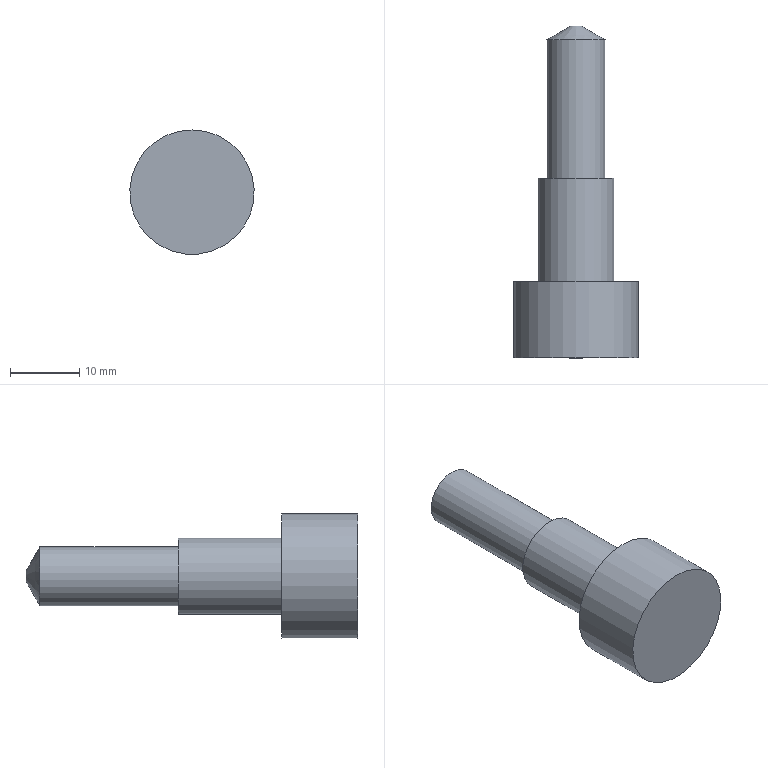Part | STEP file | solid 83 | 1 solid | 8 faces | box 18 x 48 x 18 mm | volume 5406 mm3 | plane 4 | cylinder 3 | cone 1 | commonest cylinder face diameters 8.5 x1 11 x1 18 x1